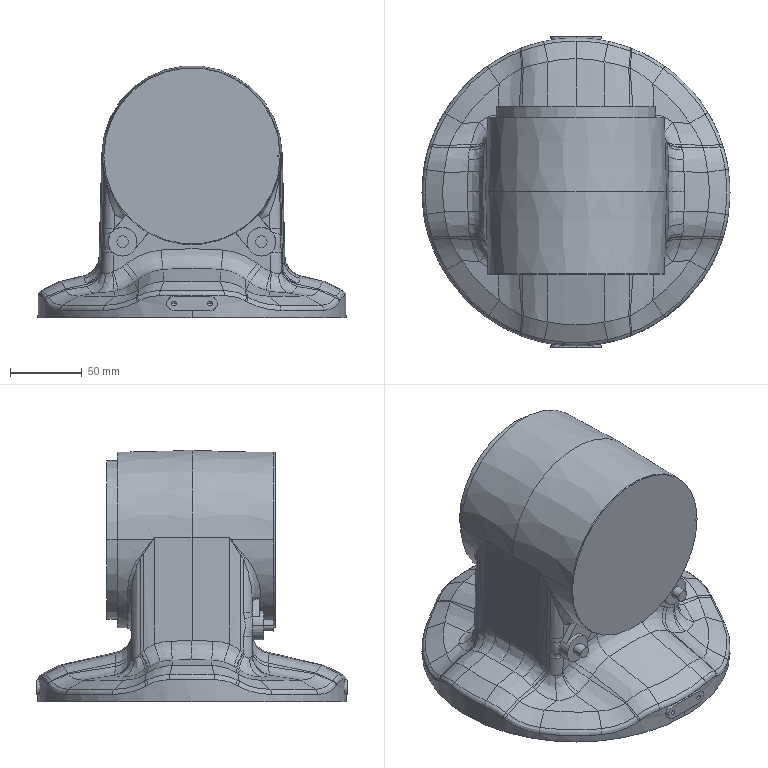Part | STEP file | ASND-0110-IRB120_3-58_IRC5_Link1_rev0 | 1 solid | 253 faces | box 215 x 217 x 176 mm | volume 2685979 mm3 | spline 135 | cylinder 37 | plane 36 | cone 34 | torus 11 | commonest cylinder face diameters 3.3 x8 16 x6 8 x4 20 x4 28 x4 64 x4